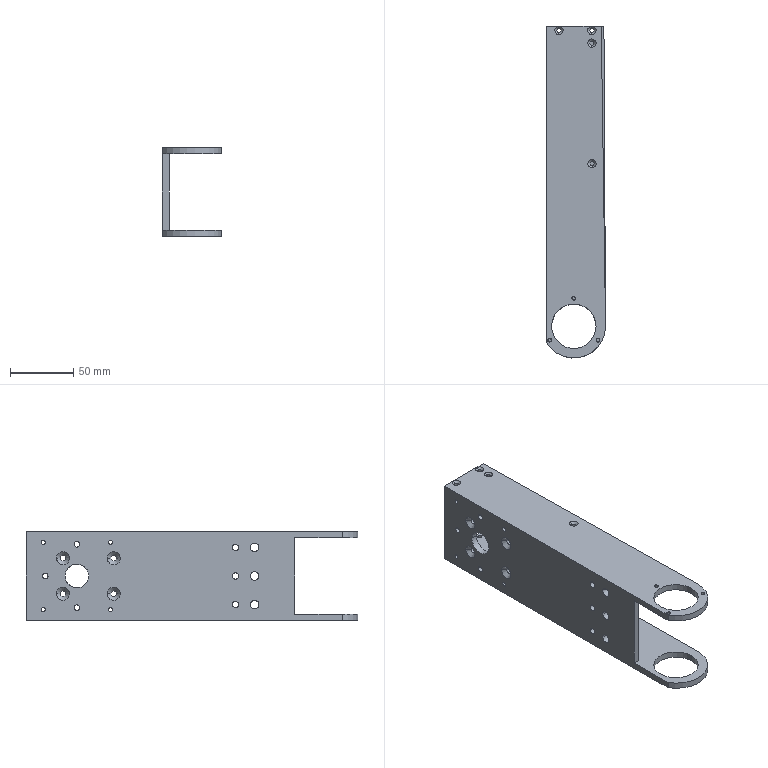Part | SolidWorks | features BaseBody 1 | 1 solid | 116 faces | box 46.554 x 261.598 x 70 mm | volume 167823 mm3 | cylinder 64 | cone 42 | plane 10 | commonest cylinder face diameters 4.5 x14 3.4 x12 3.3 x8 2.5 x6 5 x6 6.8 x6